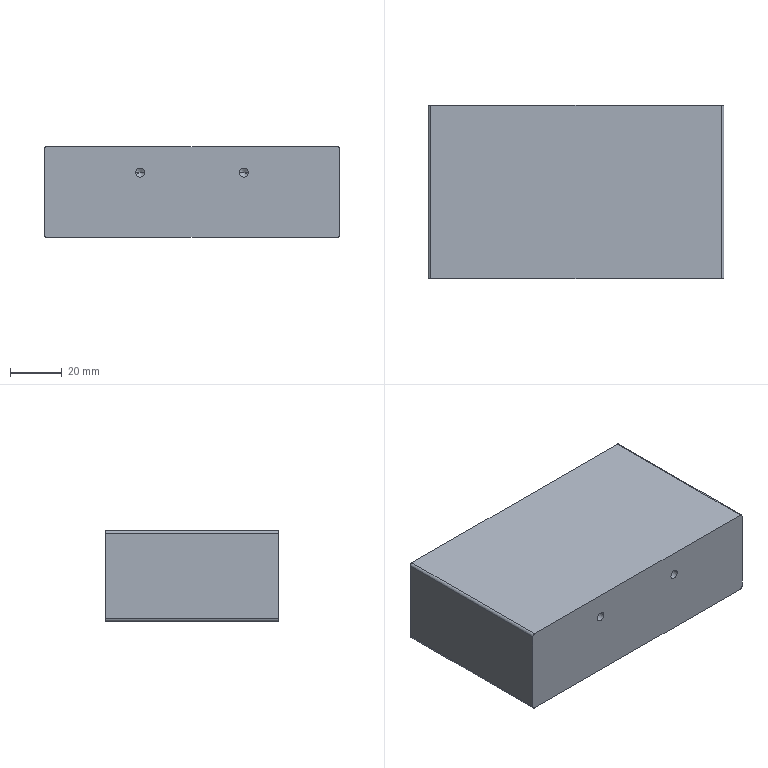Part | NX | 1 solid | 34 faces | box 114 x 67 x 35 mm | volume 266646 mm3 | cylinder 16 | cone 12 | plane 6 | commonest cylinder face diameters 3.5 x12 2 x4
STEP:
#1=CARTESIAN_POINT('',(57.,33.5,-1.));
#2=VERTEX_POINT('',#1);
#3=CARTESIAN_POINT('',(57.,33.5,-34.));
#4=VERTEX_POINT('',#3);
#5=CARTESIAN_POINT('',(57.,33.5,-1.));
#6=DIRECTION('',(0.,0.,-1.));
#7=VECTOR('',#6,1000.);
#8=LINE('',#5,#7);
#9=EDGE_CURVE('',#2,#4,#8,.T.);
#10=ORIENTED_EDGE('',*,*,#9,.T.);
#11=CARTESIAN_POINT('',(56.,33.5,-35.));
#12=VERTEX_POINT('',#11);
#13=CARTESIAN_POINT('',(56.,33.5,-34.));
#14=DIRECTION('',(0.,1.,0.));
#15=DIRECTION('',(1.,0.,0.));
#16=AXIS2_PLACEMENT_3D('',#13,#14,#15);
#17=CIRCLE('',#16,1.);
#18=EDGE_CURVE('',#4,#12,#17,.T.);
#19=ORIENTED_EDGE('',*,*,#18,.T.);
#20=CARTESIAN_POINT('',(-56.,33.5,-35.));
#21=VERTEX_POINT('',#20);
#22=CARTESIAN_POINT('',(56.,33.5,-35.));
#23=DIRECTION('',(-1.,0.,0.));
#24=VECTOR('',#23,1000.);
#25=LINE('',#22,#24);
#26=EDGE_CURVE('',#12,#21,#25,.T.);
#27=ORIENTED_EDGE('',*,*,#26,.T.);
#28=CARTESIAN_POINT('',(-57.,33.5,-34.));
#29=VERTEX_POINT('',#28);
#30=CARTESIAN_POINT('',(-56.,33.5,-34.));
#31=DIRECTION('',(0.,1.,0.));
#32=DIRECTION('',(0.,0.,-1.));
#33=AXIS2_PLACEMENT_3D('',#30,#31,#32);
#34=CIRCLE('',#33,1.);
#35=EDGE_CURVE('',#21,#29,#34,.T.);
#36=ORIENTED_EDGE('',*,*,#35,.T.);
#37=CARTESIAN_POINT('',(-57.,33.5,-1.));
#38=VERTEX_POINT('',#37);
#39=CARTESIAN_POINT('',(-57.,33.5,-34.));
#40=DIRECTION('',(0.,0.,1.));
#41=VECTOR('',#40,1000.);
#42=LINE('',#39,#41);
#43=EDGE_CURVE('',#29,#38,#42,.T.);
#44=ORIENTED_EDGE('',*,*,#43,.T.);
#45=CARTESIAN_POINT('',(-56.,33.5,0.));
#46=VERTEX_POINT('',#45);
#47=CARTESIAN_POINT('',(-56.,33.5,-1.));
#48=DIRECTION('',(0.,1.,0.));
#49=DIRECTION('',(-1.,0.,0.));
#50=AXIS2_PLACEMENT_3D('',#47,#48,#49);
#51=CIRCLE('',#50,1.);
#52=EDGE_CURVE('',#38,#46,#51,.T.);
#53=ORIENTED_EDGE('',*,*,#52,.T.);
#54=CARTESIAN_POINT('',(56.,33.5,0.));
#55=VERTEX_POINT('',#54);
#56=CARTESIAN_POINT('',(-56.,33.5,0.));
#57=DIRECTION('',(1.,0.,0.));
#58=VECTOR('',#57,1000.);
#59=LINE('',#56,#58);
#60=EDGE_CURVE('',#46,#55,#59,.T.);
#61=ORIENTED_EDGE('',*,*,#60,.T.);
#62=CARTESIAN_POINT('',(56.,33.5,-1.));
#63=DIRECTION('',(0.,1.,0.));
#64=DIRECTION('',(0.,0.,1.));
#65=AXIS2_PLACEMENT_3D('',#62,#63,#64);
#66=CIRCLE('',#65,1.);
#67=EDGE_CURVE('',#55,#2,#66,.T.);
#68=ORIENTED_EDGE('',*,*,#67,.T.);
#69=EDGE_LOOP('',(#10,#19,#27,#36,#44,#53,#61,#68));
#70=FACE_BOUND('',#69,.T.);
#71=CARTESIAN_POINT('',(15.75,33.5,-10.));
#72=VERTEX_POINT('',#71);
#73=CARTESIAN_POINT('',(19.25,33.5,-10.));
#74=VERTEX_POINT('',#73);
#75=CARTESIAN_POINT('',(17.5,33.5,-10.));
#76=DIRECTION('',(0.,1.,0.));
#77=DIRECTION('',(-1.,0.,0.));
#78=AXIS2_PLACEMENT_3D('',#75,#76,#77);
#79=CIRCLE('',#78,1.75);
#80=EDGE_CURVE('',#72,#74,#79,.T.);
#81=ORIENTED_EDGE('',*,*,#80,.F.);
#82=CARTESIAN_POINT('',(17.5,33.5,-10.));
#83=DIRECTION('',(0.,1.,0.));
#84=DIRECTION('',(1.,0.,0.));
#85=AXIS2_PLACEMENT_3D('',#82,#83,#84);
#86=CIRCLE('',#85,1.75);
#87=EDGE_CURVE('',#74,#72,#86,.T.);
#88=ORIENTED_EDGE('',*,*,#87,.F.);
#89=EDGE_LOOP('',(#81,#88));
#90=FACE_BOUND('',#89,.T.);
#91=CARTESIAN_POINT('',(50.75,33.5,-10.));
#92=VERTEX_POINT('',#91);
#93=CARTESIAN_POINT('',(54.25,33.5,-10.));
#94=VERTEX_POINT('',#93);
#95=CARTESIAN_POINT('',(52.5,33.5,-10.));
#96=DIRECTION('',(0.,1.,0.));
#97=DIRECTION('',(-1.,0.,0.));
#98=AXIS2_PLACEMENT_3D('',#95,#96,#97);
#99=CIRCLE('',#98,1.75);
#100=EDGE_CURVE('',#92,#94,#99,.T.);
#101=ORIENTED_EDGE('',*,*,#100,.F.);
#102=CARTESIAN_POINT('',(52.5,33.5,-10.));
#103=DIRECTION('',(0.,1.,0.));
#104=DIRECTION('',(1.,0.,0.));
#105=AXIS2_PLACEMENT_3D('',#102,#103,#104);
#106=CIRCLE('',#105,1.75);
#107=EDGE_CURVE('',#94,#92,#106,.T.);
#108=ORIENTED_EDGE('',*,*,#107,.F.);
#109=EDGE_LOOP('',(#101,#108));
#110=FACE_BOUND('',#109,.T.);
#111=CARTESIAN_POINT('',(-54.25,33.5,-10.));
#112=VERTEX_POINT('',#111);
#113=CARTESIAN_POINT('',(-50.75,33.5,-10.));
#114=VERTEX_POINT('',#113);
#115=CARTESIAN_POINT('',(-52.5,33.5,-10.));
#116=DIRECTION('',(0.,1.,0.));
#117=DIRECTION('',(-1.,0.,0.));
#118=AXIS2_PLACEMENT_3D('',#115,#116,#117);
#119=CIRCLE('',#118,1.75);
#120=EDGE_CURVE('',#112,#114,#119,.T.);
#121=ORIENTED_EDGE('',*,*,#120,.F.);
#122=CARTESIAN_POINT('',(-52.5,33.5,-10.));
#123=DIRECTION('',(0.,1.,0.));
#124=DIRECTION('',(1.,0.,0.));
#125=AXIS2_PLACEMENT_3D('',#122,#123,#124);
#126=CIRCLE('',#125,1.75);
#127=EDGE_CURVE('',#114,#112,#126,.T.);
#128=ORIENTED_EDGE('',*,*,#127,.F.);
#129=EDGE_LOOP('',(#121,#128));
#130=FACE_BOUND('',#129,.T.);
#131=CARTESIAN_POINT('',(-19.25,33.5,-10.));
#132=VERTEX_POINT('',#131);
#133=CARTESIAN_POINT('',(-15.75,33.5,-10.));
#134=VERTEX_POINT('',#133);
#135=CARTESIAN_POINT('',(-17.5,33.5,-10.));
#136=DIRECTION('',(0.,1.,0.));
#137=DIRECTION('',(-1.,0.,0.));
#138=AXIS2_PLACEMENT_3D('',#135,#136,#137);
#139=CIRCLE('',#138,1.75);
#140=EDGE_CURVE('',#132,#134,#139,.T.);
#141=ORIENTED_EDGE('',*,*,#140,.F.);
#142=CARTESIAN_POINT('',(-17.5,33.5,-10.));
#143=DIRECTION('',(0.,1.,0.));
#144=DIRECTION('',(1.,0.,0.));
#145=AXIS2_PLACEMENT_3D('',#142,#143,#144);
#146=CIRCLE('',#145,1.75);
#147=EDGE_CURVE('',#134,#132,#146,.T.);
#148=ORIENTED_EDGE('',*,*,#147,.F.);
#149=EDGE_LOOP('',(#141,#148));
#150=FACE_BOUND('',#149,.T.);
#151=CARTESIAN_POINT('',(0.,33.5,-10.));
#152=DIRECTION('',(0.,-1.,0.));
#153=DIRECTION('',(1.,0.,0.));
#154=AXIS2_PLACEMENT_3D('',#151,#152,#153);
#155=PLANE('',#154);
#156=ADVANCED_FACE('',(#70,#90,#110,#130,#150),#155,.F.);
#157=CARTESIAN_POINT('',(-19.25,23.,-10.));
#158=VERTEX_POINT('',#157);
#159=CARTESIAN_POINT('',(-19.25,33.5,-10.));
#160=DIRECTION('',(0.,-1.,0.));
#161=VECTOR('',#160,1000.);
#162=LINE('',#159,#161);
#163=EDGE_CURVE('',#158,#132,#162,.F.);
#164=ORIENTED_EDGE('',*,*,#163,.F.);
#165=CARTESIAN_POINT('',(-15.75,23.,-10.));
#166=VERTEX_POINT('',#165);
#167=CARTESIAN_POINT('',(-17.5,23.,-10.));
#168=DIRECTION('',(0.,-1.,0.));
#169=DIRECTION('',(-1.,0.,0.));
#170=AXIS2_PLACEMENT_3D('',#167,#168,#169);
#171=CIRCLE('',#170,1.75);
#172=EDGE_CURVE('',#158,#166,#171,.T.);
#173=ORIENTED_EDGE('',*,*,#172,.T.);
#174=CARTESIAN_POINT('',(-15.75,33.5,-10.));
#175=DIRECTION('',(0.,-1.,0.));
#176=VECTOR('',#175,1000.);
#177=LINE('',#174,#176);
#178=EDGE_CURVE('',#166,#134,#177,.F.);
#179=ORIENTED_EDGE('',*,*,#178,.T.);
#180=ORIENTED_EDGE('',*,*,#147,.T.);
#181=EDGE_LOOP('',(#164,#173,#179,#180));
#182=FACE_BOUND('',#181,.T.);
#183=CARTESIAN_POINT('',(-17.5,21.371,-10.));
#184=DIRECTION('',(0.,1.,0.));
#185=DIRECTION('',(-1.,0.,0.));
#186=AXIS2_PLACEMENT_3D('',#183,#184,#185);
#187=CYLINDRICAL_SURFACE('',#186,1.75);
#188=ADVANCED_FACE('',(#182),#187,.F.);
#189=ORIENTED_EDGE('',*,*,#178,.F.);
#190=CARTESIAN_POINT('',(-17.5,23.,-10.));
#191=DIRECTION('',(0.,-1.,0.));
#192=DIRECTION('',(1.,0.,0.));
#193=AXIS2_PLACEMENT_3D('',#190,#191,#192);
#194=CIRCLE('',#193,1.75);
#195=EDGE_CURVE('',#166,#158,#194,.T.);
#196=ORIENTED_EDGE('',*,*,#195,.T.);
#197=ORIENTED_EDGE('',*,*,#163,.T.);
#198=ORIENTED_EDGE('',*,*,#140,.T.);
#199=EDGE_LOOP('',(#189,#196,#197,#198));
#200=FACE_BOUND('',#199,.T.);
#201=CARTESIAN_POINT('',(-17.5,21.371,-10.));
#202=DIRECTION('',(0.,1.,0.));
#203=DIRECTION('',(-1.,0.,0.));
#204=AXIS2_PLACEMENT_3D('',#201,#202,#203);
#205=CYLINDRICAL_SURFACE('',#204,1.75);
#206=ADVANCED_FACE('',(#200),#205,.F.);
#207=CARTESIAN_POINT('',(-17.5,21.948,-10.));
#208=VERTEX_POINT('',#207);
#209=CARTESIAN_POINT('',(-19.25,23.,-10.));
#210=DIRECTION('',(0.8572,-0.515,0.));
#211=VECTOR('',#210,1000.);
#212=LINE('',#209,#211);
#213=EDGE_CURVE('',#158,#208,#212,.T.);
#214=ORIENTED_EDGE('',*,*,#213,.F.);
#215=ORIENTED_EDGE('',*,*,#195,.F.);
#216=CARTESIAN_POINT('',(-17.5,21.948,-10.));
#217=DIRECTION('',(0.8572,0.515,0.));
#218=VECTOR('',#217,1000.);
#219=LINE('',#216,#218);
#220=EDGE_CURVE('',#208,#166,#219,.T.);
#221=ORIENTED_EDGE('',*,*,#220,.F.);
#222=EDGE_LOOP('',(#214,#215,#221));
#223=FACE_BOUND('',#222,.T.);
#224=CARTESIAN_POINT('',(-17.5,22.474,-10.));
#225=DIRECTION('',(0.,1.,0.));
#226=DIRECTION('',(-1.,0.,0.));
#227=AXIS2_PLACEMENT_3D('',#224,#225,#226);
#228=CONICAL_SURFACE('',#227,0.875,1.03);
#229=ADVANCED_FACE('',(#223),#228,.F.);
#230=ORIENTED_EDGE('',*,*,#172,.F.);
#231=ORIENTED_EDGE('',*,*,#213,.T.);
#232=ORIENTED_EDGE('',*,*,#220,.T.);
#233=EDGE_LOOP('',(#230,#231,#232));
#234=FACE_BOUND('',#233,.T.);
#235=CARTESIAN_POINT('',(-17.5,22.474,-10.));
#236=DIRECTION('',(0.,1.,0.));
#237=DIRECTION('',(-1.,0.,0.));
#238=AXIS2_PLACEMENT_3D('',#235,#236,#237);
#239=CONICAL_SURFACE('',#238,0.875,1.03);
#240=ADVANCED_FACE('',(#234),#239,.F.);
#241=CARTESIAN_POINT('',(15.75,23.,-10.));
#242=VERTEX_POINT('',#241);
#243=CARTESIAN_POINT('',(15.75,33.5,-10.));
#244=DIRECTION('',(0.,-1.,0.));
#245=VECTOR('',#244,1000.);
#246=LINE('',#243,#245);
#247=EDGE_CURVE('',#242,#72,#246,.F.);
#248=ORIENTED_EDGE('',*,*,#247,.F.);
#249=CARTESIAN_POINT('',(19.25,23.,-10.));
#250=VERTEX_POINT('',#249);
#251=CARTESIAN_POINT('',(17.5,23.,-10.));
#252=DIRECTION('',(0.,-1.,0.));
#253=DIRECTION('',(-1.,0.,0.));
#254=AXIS2_PLACEMENT_3D('',#251,#252,#253);
#255=CIRCLE('',#254,1.75);
#256=EDGE_CURVE('',#242,#250,#255,.T.);
#257=ORIENTED_EDGE('',*,*,#256,.T.);
#258=CARTESIAN_POINT('',(19.25,33.5,-10.));
#259=DIRECTION('',(0.,-1.,0.));
#260=VECTOR('',#259,1000.);
#261=LINE('',#258,#260);
#262=EDGE_CURVE('',#250,#74,#261,.F.);
#263=ORIENTED_EDGE('',*,*,#262,.T.);
#264=ORIENTED_EDGE('',*,*,#87,.T.);
#265=EDGE_LOOP('',(#248,#257,#263,#264));
#266=FACE_BOUND('',#265,.T.);
#267=CARTESIAN_POINT('',(17.5,21.371,-10.));
#268=DIRECTION('',(0.,1.,0.));
#269=DIRECTION('',(-1.,0.,0.));
#270=AXIS2_PLACEMENT_3D('',#267,#268,#269);
#271=CYLINDRICAL_SURFACE('',#270,1.75);
#272=ADVANCED_FACE('',(#266),#271,.F.);
#273=ORIENTED_EDGE('',*,*,#262,.F.);
#274=CARTESIAN_POINT('',(17.5,23.,-10.));
#275=DIRECTION('',(0.,-1.,0.));
#276=DIRECTION('',(1.,0.,0.));
#277=AXIS2_PLACEMENT_3D('',#274,#275,#276);
#278=CIRCLE('',#277,1.75);
#279=EDGE_CURVE('',#250,#242,#278,.T.);
#280=ORIENTED_EDGE('',*,*,#279,.T.);
#281=ORIENTED_EDGE('',*,*,#247,.T.);
#282=ORIENTED_EDGE('',*,*,#80,.T.);
#283=EDGE_LOOP('',(#273,#280,#281,#282));
#284=FACE_BOUND('',#283,.T.);
#285=CARTESIAN_POINT('',(17.5,21.371,-10.));
#286=DIRECTION('',(0.,1.,0.));
#287=DIRECTION('',(-1.,0.,0.));
#288=AXIS2_PLACEMENT_3D('',#285,#286,#287);
#289=CYLINDRICAL_SURFACE('',#288,1.75);
#290=ADVANCED_FACE('',(#284),#289,.F.);
#291=CARTESIAN_POINT('',(17.5,21.948,-10.));
#292=VERTEX_POINT('',#291);
#293=CARTESIAN_POINT('',(15.75,23.,-10.));
#294=DIRECTION('',(0.8572,-0.515,0.));
#295=VECTOR('',#294,1000.);
#296=LINE('',#293,#295);
#297=EDGE_CURVE('',#292,#242,#296,.F.);
#298=ORIENTED_EDGE('',*,*,#297,.T.);
#299=ORIENTED_EDGE('',*,*,#279,.F.);
#300=CARTESIAN_POINT('',(19.25,23.,-10.));
#301=DIRECTION('',(-0.8572,-0.515,0.));
#302=VECTOR('',#301,1000.);
#303=LINE('',#300,#302);
#304=EDGE_CURVE('',#292,#250,#303,.F.);
#305=ORIENTED_EDGE('',*,*,#304,.F.);
#306=EDGE_LOOP('',(#298,#299,#305));
#307=FACE_BOUND('',#306,.T.);
#308=CARTESIAN_POINT('',(17.5,22.474,-10.));
#309=DIRECTION('',(0.,1.,0.));
#310=DIRECTION('',(-1.,0.,0.));
#311=AXIS2_PLACEMENT_3D('',#308,#309,#310);
#312=CONICAL_SURFACE('',#311,0.875,1.03);
#313=ADVANCED_FACE('',(#307),#312,.F.);
#314=ORIENTED_EDGE('',*,*,#256,.F.);
#315=ORIENTED_EDGE('',*,*,#297,.F.);
#316=ORIENTED_EDGE('',*,*,#304,.T.);
#317=EDGE_LOOP('',(#314,#315,#316));
#318=FACE_BOUND('',#317,.T.);
#319=CARTESIAN_POINT('',(17.5,22.474,-10.));
#320=DIRECTION('',(0.,1.,0.));
#321=DIRECTION('',(-1.,0.,0.));
#322=AXIS2_PLACEMENT_3D('',#319,#320,#321);
#323=CONICAL_SURFACE('',#322,0.875,1.03);
#324=ADVANCED_FACE('',(#318),#323,.F.);
#325=CARTESIAN_POINT('',(50.75,23.,-10.));
#326=VERTEX_POINT('',#325);
#327=CARTESIAN_POINT('',(50.75,33.5,-10.));
#328=DIRECTION('',(0.,-1.,0.));
#329=VECTOR('',#328,1000.);
#330=LINE('',#327,#329);
#331=EDGE_CURVE('',#326,#92,#330,.F.);
#332=ORIENTED_EDGE('',*,*,#331,.F.);
#333=CARTESIAN_POINT('',(54.25,23.,-10.));
#334=VERTEX_POINT('',#333);
#335=CARTESIAN_POINT('',(52.5,23.,-10.));
#336=DIRECTION('',(0.,-1.,0.));
#337=DIRECTION('',(-1.,0.,0.));
#338=AXIS2_PLACEMENT_3D('',#335,#336,#337);
#339=CIRCLE('',#338,1.75);
#340=EDGE_CURVE('',#326,#334,#339,.T.);
#341=ORIENTED_EDGE('',*,*,#340,.T.);
#342=CARTESIAN_POINT('',(54.25,33.5,-10.));
#343=DIRECTION('',(0.,-1.,0.));
#344=VECTOR('',#343,1000.);
#345=LINE('',#342,#344);
#346=EDGE_CURVE('',#334,#94,#345,.F.);
#347=ORIENTED_EDGE('',*,*,#346,.T.);
#348=ORIENTED_EDGE('',*,*,#107,.T.);
#349=EDGE_LOOP('',(#332,#341,#347,#348));
#350=FACE_BOUND('',#349,.T.);
#351=CARTESIAN_POINT('',(52.5,21.371,-10.));
#352=DIRECTION('',(0.,1.,0.));
#353=DIRECTION('',(-1.,0.,0.));
#354=AXIS2_PLACEMENT_3D('',#351,#352,#353);
#355=CYLINDRICAL_SURFACE('',#354,1.75);
#356=ADVANCED_FACE('',(#350),#355,.F.);
#357=ORIENTED_EDGE('',*,*,#346,.F.);
#358=CARTESIAN_POINT('',(52.5,23.,-10.));
#359=DIRECTION('',(0.,-1.,0.));
#360=DIRECTION('',(1.,0.,0.));
#361=AXIS2_PLACEMENT_3D('',#358,#359,#360);
#362=CIRCLE('',#361,1.75);
#363=EDGE_CURVE('',#334,#326,#362,.T.);
#364=ORIENTED_EDGE('',*,*,#363,.T.);
#365=ORIENTED_EDGE('',*,*,#331,.T.);
#366=ORIENTED_EDGE('',*,*,#100,.T.);
#367=EDGE_LOOP('',(#357,#364,#365,#366));
#368=FACE_BOUND('',#367,.T.);
#369=CARTESIAN_POINT('',(52.5,21.371,-10.));
#370=DIRECTION('',(0.,1.,0.));
#371=DIRECTION('',(-1.,0.,0.));
#372=AXIS2_PLACEMENT_3D('',#369,#370,#371);
#373=CYLINDRICAL_SURFACE('',#372,1.75);
#374=ADVANCED_FACE('',(#368),#373,.F.);
#375=CARTESIAN_POINT('',(52.5,21.948,-10.));
#376=VERTEX_POINT('',#375);
#377=CARTESIAN_POINT('',(50.75,23.,-10.));
#378=DIRECTION('',(0.8572,-0.515,0.));
#379=VECTOR('',#378,1000.);
#380=LINE('',#377,#379);
#381=EDGE_CURVE('',#376,#326,#380,.F.);
#382=ORIENTED_EDGE('',*,*,#381,.T.);
#383=ORIENTED_EDGE('',*,*,#363,.F.);
#384=CARTESIAN_POINT('',(54.25,23.,-10.));
#385=DIRECTION('',(-0.8572,-0.515,0.));
#386=VECTOR('',#385,1000.);
#387=LINE('',#384,#386);
#388=EDGE_CURVE('',#376,#334,#387,.F.);
#389=ORIENTED_EDGE('',*,*,#388,.F.);
#390=EDGE_LOOP('',(#382,#383,#389));
#391=FACE_BOUND('',#390,.T.);
#392=CARTESIAN_POINT('',(52.5,22.474,-10.));
#393=DIRECTION('',(0.,1.,0.));
#394=DIRECTION('',(-1.,0.,0.));
#395=AXIS2_PLACEMENT_3D('',#392,#393,#394);
#396=CONICAL_SURFACE('',#395,0.875,1.03);
#397=ADVANCED_FACE('',(#391),#396,.F.);
#398=ORIENTED_EDGE('',*,*,#340,.F.);
#399=ORIENTED_EDGE('',*,*,#381,.F.);
#400=ORIENTED_EDGE('',*,*,#388,.T.);
#401=EDGE_LOOP('',(#398,#399,#400));
#402=FACE_BOUND('',#401,.T.);
#403=CARTESIAN_POINT('',(52.5,22.474,-10.));
#404=DIRECTION('',(0.,1.,0.));
#405=DIRECTION('',(-1.,0.,0.));
#406=AXIS2_PLACEMENT_3D('',#403,#404,#405);
#407=CONICAL_SURFACE('',#406,0.875,1.03);
#408=ADVANCED_FACE('',(#402),#407,.F.);
#409=CARTESIAN_POINT('',(-54.25,23.,-10.));
#410=VERTEX_POINT('',#409);
#411=CARTESIAN_POINT('',(-54.25,33.5,-10.));
#412=DIRECTION('',(0.,-1.,0.));
#413=VECTOR('',#412,1000.);
#414=LINE('',#411,#413);
#415=EDGE_CURVE('',#410,#112,#414,.F.);
#416=ORIENTED_EDGE('',*,*,#415,.F.);
#417=CARTESIAN_POINT('',(-50.75,23.,-10.));
#418=VERTEX_POINT('',#417);
#419=CARTESIAN_POINT('',(-52.5,23.,-10.));
#420=DIRECTION('',(0.,-1.,0.));
#421=DIRECTION('',(-1.,0.,0.));
#422=AXIS2_PLACEMENT_3D('',#419,#420,#421);
#423=CIRCLE('',#422,1.75);
#424=EDGE_CURVE('',#410,#418,#423,.T.);
#425=ORIENTED_EDGE('',*,*,#424,.T.);
#426=CARTESIAN_POINT('',(-50.75,33.5,-10.));
#427=DIRECTION('',(0.,-1.,0.));
#428=VECTOR('',#427,1000.);
#429=LINE('',#426,#428);
#430=EDGE_CURVE('',#418,#114,#429,.F.);
#431=ORIENTED_EDGE('',*,*,#430,.T.);
#432=ORIENTED_EDGE('',*,*,#127,.T.);
#433=EDGE_LOOP('',(#416,#425,#431,#432));
#434=FACE_BOUND('',#433,.T.);
#435=CARTESIAN_POINT('',(-52.5,21.371,-10.));
#436=DIRECTION('',(0.,1.,0.));
#437=DIRECTION('',(-1.,0.,0.));
#438=AXIS2_PLACEMENT_3D('',#435,#436,#437);
#439=CYLINDRICAL_SURFACE('',#438,1.75);
#440=ADVANCED_FACE('',(#434),#439,.F.);
#441=ORIENTED_EDGE('',*,*,#430,.F.);
#442=CARTESIAN_POINT('',(-52.5,23.,-10.));
#443=DIRECTION('',(0.,-1.,0.));
#444=DIRECTION('',(1.,0.,0.));
#445=AXIS2_PLACEMENT_3D('',#442,#443,#444);
#446=CIRCLE('',#445,1.75);
#447=EDGE_CURVE('',#418,#410,#446,.T.);
#448=ORIENTED_EDGE('',*,*,#447,.T.);
#449=ORIENTED_EDGE('',*,*,#415,.T.);
#450=ORIENTED_EDGE('',*,*,#120,.T.);
#451=EDGE_LOOP('',(#441,#448,#449,#450));
#452=FACE_BOUND('',#451,.T.);
#453=CARTESIAN_POINT('',(-52.5,21.371,-10.));
#454=DIRECTION('',(0.,1.,0.));
#455=DIRECTION('',(-1.,0.,0.));
#456=AXIS2_PLACEMENT_3D('',#453,#454,#455);
#457=CYLINDRICAL_SURFACE('',#456,1.75);
#458=ADVANCED_FACE('',(#452),#457,.F.);
#459=CARTESIAN_POINT('',(-52.5,21.948,-10.));
#460=VERTEX_POINT('',#459);
#461=CARTESIAN_POINT('',(-54.25,23.,-10.));
#462=DIRECTION('',(0.8572,-0.515,0.));
#463=VECTOR('',#462,1000.);
#464=LINE('',#461,#463);
#465=EDGE_CURVE('',#410,#460,#464,.T.);
#466=ORIENTED_EDGE('',*,*,#465,.F.);
#467=ORIENTED_EDGE('',*,*,#447,.F.);
#468=CARTESIAN_POINT('',(-52.5,21.948,-10.));
#469=DIRECTION('',(0.8572,0.515,0.));
#470=VECTOR('',#469,1000.);
#471=LINE('',#468,#470);
#472=EDGE_CURVE('',#460,#418,#471,.T.);
#473=ORIENTED_EDGE('',*,*,#472,.F.);
#474=EDGE_LOOP('',(#466,#467,#473));
#475=FACE_BOUND('',#474,.T.);
#476=CARTESIAN_POINT('',(-52.5,22.474,-10.));
#477=DIRECTION('',(0.,1.,0.));
#478=DIRECTION('',(-1.,0.,0.));
#479=AXIS2_PLACEMENT_3D('',#476,#477,#478);
#480=CONICAL_SURFACE('',#479,0.875,1.03);
#481=ADVANCED_FACE('',(#475),#480,.F.);
#482=ORIENTED_EDGE('',*,*,#424,.F.);
#483=ORIENTED_EDGE('',*,*,#465,.T.);
#484=ORIENTED_EDGE('',*,*,#472,.T.);
#485=EDGE_LOOP('',(#482,#483,#484));
#486=FACE_BOUND('',#485,.T.);
#487=CARTESIAN_POINT('',(-52.5,22.474,-10.));
#488=DIRECTION('',(0.,1.,0.));
#489=DIRECTION('',(-1.,0.,0.));
#490=AXIS2_PLACEMENT_3D('',#487,#488,#489);
#491=CONICAL_SURFACE('',#490,0.875,1.03);
#492=ADVANCED_FACE('',(#486),#491,.F.);
#493=CARTESIAN_POINT('',(56.,-33.5,0.));
#494=VERTEX_POINT('',#493);
#495=CARTESIAN_POINT('',(56.,-33.5,0.));
#496=DIRECTION('',(0.,1.,0.));
#497=VECTOR('',#496,1000.);
#498=LINE('',#495,#497);
#499=EDGE_CURVE('',#494,#55,#498,.T.);
#500=ORIENTED_EDGE('',*,*,#499,.F.);
#501=CARTESIAN_POINT('',(57.,-33.5,-1.));
#502=VERTEX_POINT('',#501);
#503=CARTESIAN_POINT('',(56.,-33.5,-1.));
#504=DIRECTION('',(0.,-1.,0.));
#505=DIRECTION('',(1.,0.,0.));
#506=AXIS2_PLACEMENT_3D('',#503,#504,#505);
#507=CIRCLE('',#506,1.);
#508=EDGE_CURVE('',#502,#494,#507,.T.);
#509=ORIENTED_EDGE('',*,*,#508,.F.);
#510=CARTESIAN_POINT('',(57.,-33.5,-1.));
#511=DIRECTION('',(0.,1.,0.));
#512=VECTOR('',#511,1000.);
#513=LINE('',#510,#512);
#514=EDGE_CURVE('',#502,#2,#513,.T.);
#515=ORIENTED_EDGE('',*,*,#514,.T.);
#516=ORIENTED_EDGE('',*,*,#67,.F.);
#517=EDGE_LOOP('',(#500,#509,#515,#516));
#518=FACE_BOUND('',#517,.T.);
#519=CARTESIAN_POINT('',(56.,-120.841,-1.));
#520=DIRECTION('',(0.,1.,0.));
#521=DIRECTION('',(0.,0.,-1.));
#522=AXIS2_PLACEMENT_3D('',#519,#520,#521);
#523=CYLINDRICAL_SURFACE('',#522,1.);
#524=ADVANCED_FACE('',(#518),#523,.T.);
#525=CARTESIAN_POINT('',(57.,-33.5,-34.));
#526=VERTEX_POINT('',#525);
#527=CARTESIAN_POINT('',(57.,-33.5,-34.));
#528=DIRECTION('',(0.,0.,1.));
#529=VECTOR('',#528,1000.);
#530=LINE('',#527,#529);
#531=EDGE_CURVE('',#526,#502,#530,.T.);
#532=ORIENTED_EDGE('',*,*,#531,.F.);
#533=CARTESIAN_POINT('',(57.,-33.5,-34.));
#534=DIRECTION('',(0.,1.,0.));
#535=VECTOR('',#534,1000.);
#536=LINE('',#533,#535);
#537=EDGE_CURVE('',#526,#4,#536,.T.);
#538=ORIENTED_EDGE('',*,*,#537,.T.);
#539=ORIENTED_EDGE('',*,*,#9,.F.);
#540=ORIENTED_EDGE('',*,*,#514,.F.);
#541=EDGE_LOOP('',(#532,#538,#539,#540));
#542=FACE_BOUND('',#541,.T.);
#543=CARTESIAN_POINT('',(57.,33.5,-20.));
#544=DIRECTION('',(1.,0.,0.));
#545=DIRECTION('',(0.,0.,-1.));
#546=AXIS2_PLACEMENT_3D('',#543,#544,#545);
#547=PLANE('',#546);
#548=ADVANCED_FACE('',(#542),#547,.T.);
#549=ORIENTED_EDGE('',*,*,#537,.F.);
#550=CARTESIAN_POINT('',(56.,-33.5,-35.));
#551=VERTEX_POINT('',#550);
#552=CARTESIAN_POINT('',(56.,-33.5,-34.));
#553=DIRECTION('',(0.,-1.,0.));
#554=DIRECTION('',(0.,0.,-1.));
#555=AXIS2_PLACEMENT_3D('',#552,#553,#554);
#556=CIRCLE('',#555,1.);
#557=EDGE_CURVE('',#551,#526,#556,.T.);
#558=ORIENTED_EDGE('',*,*,#557,.F.);
#559=CARTESIAN_POINT('',(56.,-33.5,-35.));
#560=DIRECTION('',(0.,1.,0.));
#561=VECTOR('',#560,1000.);
#562=LINE('',#559,#561);
#563=EDGE_CURVE('',#551,#12,#562,.T.);
#564=ORIENTED_EDGE('',*,*,#563,.T.);
#565=ORIENTED_EDGE('',*,*,#18,.F.);
#566=EDGE_LOOP('',(#549,#558,#564,#565));
#567=FACE_BOUND('',#566,.T.);
#568=CARTESIAN_POINT('',(56.,-120.841,-34.));
#569=DIRECTION('',(0.,1.,0.));
#570=DIRECTION('',(-1.,0.,0.));
#571=AXIS2_PLACEMENT_3D('',#568,#569,#570);
#572=CYLINDRICAL_SURFACE('',#571,1.);
#573=ADVANCED_FACE('',(#567),#572,.T.);
#574=CARTESIAN_POINT('',(-56.,-33.5,-35.));
#575=VERTEX_POINT('',#574);
#576=CARTESIAN_POINT('',(-56.,-33.5,-35.));
#577=DIRECTION('',(1.,0.,0.));
#578=VECTOR('',#577,1000.);
#579=LINE('',#576,#578);
#580=EDGE_CURVE('',#575,#551,#579,.T.);
#581=ORIENTED_EDGE('',*,*,#580,.F.);
#582=CARTESIAN_POINT('',(-56.,-33.5,-35.));
#583=DIRECTION('',(0.,1.,0.));
#584=VECTOR('',#583,1000.);
#585=LINE('',#582,#584);
#586=EDGE_CURVE('',#575,#21,#585,.T.);
#587=ORIENTED_EDGE('',*,*,#586,.T.);
#588=ORIENTED_EDGE('',*,*,#26,.F.);
#589=ORIENTED_EDGE('',*,*,#563,.F.);
#590=EDGE_LOOP('',(#581,#587,#588,#589));
#591=FACE_BOUND('',#590,.T.);
#592=CARTESIAN_POINT('',(-60.,33.5,-35.));
#593=DIRECTION('',(0.,0.,-1.));
#594=DIRECTION('',(-1.,0.,0.));
#595=AXIS2_PLACEMENT_3D('',#592,#593,#594);
#596=PLANE('',#595);
#597=ADVANCED_FACE('',(#591),#596,.T.);
#598=ORIENTED_EDGE('',*,*,#586,.F.);
#599=CARTESIAN_POINT('',(-57.,-33.5,-34.));
#600=VERTEX_POINT('',#599);
#601=CARTESIAN_POINT('',(-56.,-33.5,-34.));
#602=DIRECTION('',(0.,-1.,0.));
#603=DIRECTION('',(-1.,0.,0.));
#604=AXIS2_PLACEMENT_3D('',#601,#602,#603);
#605=CIRCLE('',#604,1.);
#606=EDGE_CURVE('',#600,#575,#605,.T.);
#607=ORIENTED_EDGE('',*,*,#606,.F.);
#608=CARTESIAN_POINT('',(-57.,-33.5,-34.));
#609=DIRECTION('',(0.,1.,0.));
#610=VECTOR('',#609,1000.);
#611=LINE('',#608,#610);
#612=EDGE_CURVE('',#600,#29,#611,.T.);
#613=ORIENTED_EDGE('',*,*,#612,.T.);
#614=ORIENTED_EDGE('',*,*,#35,.F.);
#615=EDGE_LOOP('',(#598,#607,#613,#614));
#616=FACE_BOUND('',#615,.T.);
#617=CARTESIAN_POINT('',(-56.,-120.841,-34.));
#618=DIRECTION('',(0.,1.,0.));
#619=DIRECTION('',(0.,0.,1.));
#620=AXIS2_PLACEMENT_3D('',#617,#618,#619);
#621=CYLINDRICAL_SURFACE('',#620,1.);
#622=ADVANCED_FACE('',(#616),#621,.T.);
#623=ORIENTED_EDGE('',*,*,#43,.F.);
#624=ORIENTED_EDGE('',*,*,#612,.F.);
#625=CARTESIAN_POINT('',(-57.,-33.5,-1.));
#626=VERTEX_POINT('',#625);
#627=CARTESIAN_POINT('',(-57.,-33.5,-34.));
#628=DIRECTION('',(0.,0.,1.));
#629=VECTOR('',#628,1000.);
#630=LINE('',#627,#629);
#631=EDGE_CURVE('',#600,#626,#630,.T.);
#632=ORIENTED_EDGE('',*,*,#631,.T.);
#633=CARTESIAN_POINT('',(-57.,-33.5,-1.));
#634=DIRECTION('',(0.,1.,0.));
#635=VECTOR('',#634,1000.);
#636=LINE('',#633,#635);
#637=EDGE_CURVE('',#626,#38,#636,.T.);
#638=ORIENTED_EDGE('',*,*,#637,.T.);
#639=EDGE_LOOP('',(#623,#624,#632,#638));
#640=FACE_BOUND('',#639,.T.);
#641=CARTESIAN_POINT('',(-57.,33.5,0.));
#642=DIRECTION('',(-1.,0.,0.));
#643=DIRECTION('',(0.,0.,1.));
#644=AXIS2_PLACEMENT_3D('',#641,#642,#643);
#645=PLANE('',#644);
#646=ADVANCED_FACE('',(#640),#645,.T.);
#647=ORIENTED_EDGE('',*,*,#637,.F.);
#648=CARTESIAN_POINT('',(-56.,-33.5,0.));
#649=VERTEX_POINT('',#648);
#650=CARTESIAN_POINT('',(-56.,-33.5,-1.));
#651=DIRECTION('',(0.,-1.,0.));
#652=DIRECTION('',(0.,0.,1.));
#653=AXIS2_PLACEMENT_3D('',#650,#651,#652);
#654=CIRCLE('',#653,1.);
#655=EDGE_CURVE('',#649,#626,#654,.T.);
#656=ORIENTED_EDGE('',*,*,#655,.F.);
#657=CARTESIAN_POINT('',(-56.,-33.5,0.));
#658=DIRECTION('',(0.,1.,0.));
#659=VECTOR('',#658,1000.);
#660=LINE('',#657,#659);
#661=EDGE_CURVE('',#649,#46,#660,.T.);
#662=ORIENTED_EDGE('',*,*,#661,.T.);
#663=ORIENTED_EDGE('',*,*,#52,.F.);
#664=EDGE_LOOP('',(#647,#656,#662,#663));
#665=FACE_BOUND('',#664,.T.);
#666=CARTESIAN_POINT('',(-56.,-120.841,-1.));
#667=DIRECTION('',(0.,1.,0.));
#668=DIRECTION('',(1.,0.,0.));
#669=AXIS2_PLACEMENT_3D('',#666,#667,#668);
#670=CYLINDRICAL_SURFACE('',#669,1.);
#671=ADVANCED_FACE('',(#665),#670,.T.);
#672=ORIENTED_EDGE('',*,*,#60,.F.);
#673=ORIENTED_EDGE('',*,*,#661,.F.);
#674=CARTESIAN_POINT('',(56.,-33.5,0.));
#675=DIRECTION('',(-1.,0.,0.));
#676=VECTOR('',#675,1000.);
#677=LINE('',#674,#676);
#678=EDGE_CURVE('',#494,#649,#677,.T.);
#679=ORIENTED_EDGE('',*,*,#678,.F.);
#680=ORIENTED_EDGE('',*,*,#499,.T.);
#681=EDGE_LOOP('',(#672,#673,#679,#680));
#682=FACE_BOUND('',#681,.T.);
#683=CARTESIAN_POINT('',(60.,33.5,0.));
#684=DIRECTION('',(0.,0.,1.));
#685=DIRECTION('',(1.,0.,0.));
#686=AXIS2_PLACEMENT_3D('',#683,#684,#685);
#687=PLANE('',#686);
#688=ADVANCED_FACE('',(#682),#687,.T.);
#689=ORIENTED_EDGE('',*,*,#678,.T.);
#690=ORIENTED_EDGE('',*,*,#655,.T.);
#691=ORIENTED_EDGE('',*,*,#631,.F.);
#692=ORIENTED_EDGE('',*,*,#606,.T.);
#693=ORIENTED_EDGE('',*,*,#580,.T.);
#694=ORIENTED_EDGE('',*,*,#557,.T.);
#695=ORIENTED_EDGE('',*,*,#531,.T.);
#696=ORIENTED_EDGE('',*,*,#508,.T.);
#697=EDGE_LOOP('',(#689,#690,#691,#692,#693,#694,#695,#696));
#698=FACE_BOUND('',#697,.T.);
#699=CARTESIAN_POINT('',(-18.25,-33.5,-10.));
#700=VERTEX_POINT('',#699);
#701=CARTESIAN_POINT('',(-21.75,-33.5,-10.));
#702=VERTEX_POINT('',#701);
#703=CARTESIAN_POINT('',(-20.,-33.5,-10.));
#704=DIRECTION('',(0.,-1.,0.));
#705=DIRECTION('',(1.,0.,0.));
#706=AXIS2_PLACEMENT_3D('',#703,#704,#705);
#707=CIRCLE('',#706,1.75);
#708=EDGE_CURVE('',#700,#702,#707,.T.);
#709=ORIENTED_EDGE('',*,*,#708,.F.);
#710=CARTESIAN_POINT('',(-20.,-33.5,-10.));
#711=DIRECTION('',(0.,-1.,0.));
#712=DIRECTION('',(-1.,0.,0.));
#713=AXIS2_PLACEMENT_3D('',#710,#711,#712);
#714=CIRCLE('',#713,1.75);
#715=EDGE_CURVE('',#702,#700,#714,.T.);
#716=ORIENTED_EDGE('',*,*,#715,.F.);
#717=EDGE_LOOP('',(#709,#716));
#718=FACE_BOUND('',#717,.T.);
#719=CARTESIAN_POINT('',(21.75,-33.5,-10.));
#720=VERTEX_POINT('',#719);
#721=CARTESIAN_POINT('',(18.25,-33.5,-10.));
#722=VERTEX_POINT('',#721);
#723=CARTESIAN_POINT('',(20.,-33.5,-10.));
#724=DIRECTION('',(0.,-1.,0.));
#725=DIRECTION('',(1.,0.,0.));
#726=AXIS2_PLACEMENT_3D('',#723,#724,#725);
#727=CIRCLE('',#726,1.75);
#728=EDGE_CURVE('',#720,#722,#727,.T.);
#729=ORIENTED_EDGE('',*,*,#728,.F.);
#730=CARTESIAN_POINT('',(20.,-33.5,-10.));
#731=DIRECTION('',(0.,-1.,0.));
#732=DIRECTION('',(-1.,0.,0.));
#733=AXIS2_PLACEMENT_3D('',#730,#731,#732);
#734=CIRCLE('',#733,1.75);
#735=EDGE_CURVE('',#722,#720,#734,.T.);
#736=ORIENTED_EDGE('',*,*,#735,.F.);
#737=EDGE_LOOP('',(#729,#736));
#738=FACE_BOUND('',#737,.T.);
#739=CARTESIAN_POINT('',(0.,-33.5,-10.));
#740=DIRECTION('',(0.,-1.,0.));
#741=DIRECTION('',(1.,0.,0.));
#742=AXIS2_PLACEMENT_3D('',#739,#740,#741);
#743=PLANE('',#742);
#744=ADVANCED_FACE('',(#698,#718,#738),#743,.T.);
#745=CARTESIAN_POINT('',(21.75,-23.,-10.));
#746=VERTEX_POINT('',#745);
#747=CARTESIAN_POINT('',(21.75,-33.5,-10.));
#748=DIRECTION('',(0.,1.,0.));
#749=VECTOR('',#748,1000.);
#750=LINE('',#747,#749);
#751=EDGE_CURVE('',#746,#720,#750,.F.);
#752=ORIENTED_EDGE('',*,*,#751,.F.);
#753=CARTESIAN_POINT('',(18.25,-23.,-10.));
#754=VERTEX_POINT('',#753);
#755=CARTESIAN_POINT('',(20.,-23.,-10.));
#756=DIRECTION('',(0.,1.,0.));
#757=DIRECTION('',(1.,0.,0.));
#758=AXIS2_PLACEMENT_3D('',#755,#756,#757);
#759=CIRCLE('',#758,1.75);
#760=EDGE_CURVE('',#746,#754,#759,.T.);
#761=ORIENTED_EDGE('',*,*,#760,.T.);
#762=CARTESIAN_POINT('',(18.25,-33.5,-10.));
#763=DIRECTION('',(0.,1.,0.));
#764=VECTOR('',#763,1000.);
#765=LINE('',#762,#764);
#766=EDGE_CURVE('',#754,#722,#765,.F.);
#767=ORIENTED_EDGE('',*,*,#766,.T.);
#768=ORIENTED_EDGE('',*,*,#735,.T.);
#769=EDGE_LOOP('',(#752,#761,#767,#768));
#770=FACE_BOUND('',#769,.T.);
#771=CARTESIAN_POINT('',(20.,-21.371,-10.));
#772=DIRECTION('',(0.,-1.,0.));
#773=DIRECTION('',(1.,0.,0.));
#774=AXIS2_PLACEMENT_3D('',#771,#772,#773);
#775=CYLINDRICAL_SURFACE('',#774,1.75);
#776=ADVANCED_FACE('',(#770),#775,.F.);
#777=ORIENTED_EDGE('',*,*,#766,.F.);
#778=CARTESIAN_POINT('',(20.,-23.,-10.));
#779=DIRECTION('',(0.,1.,0.));
#780=DIRECTION('',(-1.,0.,0.));
#781=AXIS2_PLACEMENT_3D('',#778,#779,#780);
#782=CIRCLE('',#781,1.75);
#783=EDGE_CURVE('',#754,#746,#782,.T.);
#784=ORIENTED_EDGE('',*,*,#783,.T.);
#785=ORIENTED_EDGE('',*,*,#751,.T.);
#786=ORIENTED_EDGE('',*,*,#728,.T.);
#787=EDGE_LOOP('',(#777,#784,#785,#786));
#788=FACE_BOUND('',#787,.T.);
#789=CARTESIAN_POINT('',(20.,-21.371,-10.));
#790=DIRECTION('',(0.,-1.,0.));
#791=DIRECTION('',(1.,0.,0.));
#792=AXIS2_PLACEMENT_3D('',#789,#790,#791);
#793=CYLINDRICAL_SURFACE('',#792,1.75);
#794=ADVANCED_FACE('',(#788),#793,.F.);
#795=CARTESIAN_POINT('',(20.,-21.948,-10.));
#796=VERTEX_POINT('',#795);
#797=CARTESIAN_POINT('',(21.75,-23.,-10.));
#798=DIRECTION('',(-0.8572,0.515,0.));
#799=VECTOR('',#798,1000.);
#800=LINE('',#797,#799);
#801=EDGE_CURVE('',#746,#796,#800,.T.);
#802=ORIENTED_EDGE('',*,*,#801,.F.);
#803=ORIENTED_EDGE('',*,*,#783,.F.);
#804=CARTESIAN_POINT('',(20.,-21.948,-10.));
#805=DIRECTION('',(-0.8572,-0.515,0.));
#806=VECTOR('',#805,1000.);
#807=LINE('',#804,#806);
#808=EDGE_CURVE('',#796,#754,#807,.T.);
#809=ORIENTED_EDGE('',*,*,#808,.F.);
#810=EDGE_LOOP('',(#802,#803,#809));
#811=FACE_BOUND('',#810,.T.);
#812=CARTESIAN_POINT('',(20.,-22.474,-10.));
#813=DIRECTION('',(0.,-1.,0.));
#814=DIRECTION('',(1.,0.,0.));
#815=AXIS2_PLACEMENT_3D('',#812,#813,#814);
#816=CONICAL_SURFACE('',#815,0.875,1.03);
#817=ADVANCED_FACE('',(#811),#816,.F.);
#818=ORIENTED_EDGE('',*,*,#760,.F.);
#819=ORIENTED_EDGE('',*,*,#801,.T.);
#820=ORIENTED_EDGE('',*,*,#808,.T.);
#821=EDGE_LOOP('',(#818,#819,#820));
#822=FACE_BOUND('',#821,.T.);
#823=CARTESIAN_POINT('',(20.,-22.474,-10.));
#824=DIRECTION('',(0.,-1.,0.));
#825=DIRECTION('',(1.,0.,0.));
#826=AXIS2_PLACEMENT_3D('',#823,#824,#825);
#827=CONICAL_SURFACE('',#826,0.875,1.03);
#828=ADVANCED_FACE('',(#822),#827,.F.);
#829=CARTESIAN_POINT('',(-18.25,-23.,-10.));
#830=VERTEX_POINT('',#829);
#831=CARTESIAN_POINT('',(-18.25,-33.5,-10.));
#832=DIRECTION('',(0.,1.,0.));
#833=VECTOR('',#832,1000.);
#834=LINE('',#831,#833);
#835=EDGE_CURVE('',#830,#700,#834,.F.);
#836=ORIENTED_EDGE('',*,*,#835,.F.);
#837=CARTESIAN_POINT('',(-21.75,-23.,-10.));
#838=VERTEX_POINT('',#837);
#839=CARTESIAN_POINT('',(-20.,-23.,-10.));
#840=DIRECTION('',(0.,1.,0.));
#841=DIRECTION('',(1.,0.,0.));
#842=AXIS2_PLACEMENT_3D('',#839,#840,#841);
#843=CIRCLE('',#842,1.75);
#844=EDGE_CURVE('',#830,#838,#843,.T.);
#845=ORIENTED_EDGE('',*,*,#844,.T.);
#846=CARTESIAN_POINT('',(-21.75,-33.5,-10.));
#847=DIRECTION('',(0.,1.,0.));
#848=VECTOR('',#847,1000.);
#849=LINE('',#846,#848);
#850=EDGE_CURVE('',#838,#702,#849,.F.);
#851=ORIENTED_EDGE('',*,*,#850,.T.);
#852=ORIENTED_EDGE('',*,*,#715,.T.);
#853=EDGE_LOOP('',(#836,#845,#851,#852));
#854=FACE_BOUND('',#853,.T.);
#855=CARTESIAN_POINT('',(-20.,-21.371,-10.));
#856=DIRECTION('',(0.,-1.,0.));
#857=DIRECTION('',(1.,0.,0.));
#858=AXIS2_PLACEMENT_3D('',#855,#856,#857);
#859=CYLINDRICAL_SURFACE('',#858,1.75);
#860=ADVANCED_FACE('',(#854),#859,.F.);
#861=ORIENTED_EDGE('',*,*,#850,.F.);
#862=CARTESIAN_POINT('',(-20.,-23.,-10.));
#863=DIRECTION('',(0.,1.,0.));
#864=DIRECTION('',(-1.,0.,0.));
#865=AXIS2_PLACEMENT_3D('',#862,#863,#864);
#866=CIRCLE('',#865,1.75);
#867=EDGE_CURVE('',#838,#830,#866,.T.);
#868=ORIENTED_EDGE('',*,*,#867,.T.);
#869=ORIENTED_EDGE('',*,*,#835,.T.);
#870=ORIENTED_EDGE('',*,*,#708,.T.);
#871=EDGE_LOOP('',(#861,#868,#869,#870));
#872=FACE_BOUND('',#871,.T.);
#873=CARTESIAN_POINT('',(-20.,-21.371,-10.));
#874=DIRECTION('',(0.,-1.,0.));
#875=DIRECTION('',(1.,0.,0.));
#876=AXIS2_PLACEMENT_3D('',#873,#874,#875);
#877=CYLINDRICAL_SURFACE('',#876,1.75);
#878=ADVANCED_FACE('',(#872),#877,.F.);
#879=CARTESIAN_POINT('',(-20.,-21.948,-10.));
#880=VERTEX_POINT('',#879);
#881=CARTESIAN_POINT('',(-18.25,-23.,-10.));
#882=DIRECTION('',(-0.8572,0.515,0.));
#883=VECTOR('',#882,1000.);
#884=LINE('',#881,#883);
#885=EDGE_CURVE('',#830,#880,#884,.T.);
#886=ORIENTED_EDGE('',*,*,#885,.F.);
#887=ORIENTED_EDGE('',*,*,#867,.F.);
#888=CARTESIAN_POINT('',(-20.,-21.948,-10.));
#889=DIRECTION('',(-0.8572,-0.515,0.));
#890=VECTOR('',#889,1000.);
#891=LINE('',#888,#890);
#892=EDGE_CURVE('',#880,#838,#891,.T.);
#893=ORIENTED_EDGE('',*,*,#892,.F.);
#894=EDGE_LOOP('',(#886,#887,#893));
#895=FACE_BOUND('',#894,.T.);
#896=CARTESIAN_POINT('',(-20.,-22.474,-10.));
#897=DIRECTION('',(0.,-1.,0.));
#898=DIRECTION('',(1.,0.,0.));
#899=AXIS2_PLACEMENT_3D('',#896,#897,#898);
#900=CONICAL_SURFACE('',#899,0.875,1.03);
#901=ADVANCED_FACE('',(#895),#900,.F.);
#902=ORIENTED_EDGE('',*,*,#844,.F.);
#903=ORIENTED_EDGE('',*,*,#885,.T.);
#904=ORIENTED_EDGE('',*,*,#892,.T.);
#905=EDGE_LOOP('',(#902,#903,#904));
#906=FACE_BOUND('',#905,.T.);
#907=CARTESIAN_POINT('',(-20.,-22.474,-10.));
#908=DIRECTION('',(0.,-1.,0.));
#909=DIRECTION('',(1.,0.,0.));
#910=AXIS2_PLACEMENT_3D('',#907,#908,#909);
#911=CONICAL_SURFACE('',#910,0.875,1.03);
#912=ADVANCED_FACE('',(#906),#911,.F.);
#913=CLOSED_SHELL('',(#156,#188,#206,#229,#240,#272,#290,#313,#324,#356,#374,#397,#408,#440,#458,#481,#492,#524,#548,#573,#597,#622,#646,#671,#688,#744,#776,#794,#817,#828,#860,#878,#901,#912));
#914=MANIFOLD_SOLID_BREP('',#913);
#915=(LENGTH_UNIT()NAMED_UNIT(*)SI_UNIT(.MILLI.,.METRE.));
#916=UNCERTAINTY_MEASURE_WITH_UNIT(LENGTH_MEASURE(0.00001),#915,'','');
#917=(NAMED_UNIT(*)PLANE_ANGLE_UNIT()SI_UNIT($,.RADIAN.));
#918=(NAMED_UNIT(*)SI_UNIT($,.STERADIAN.)SOLID_ANGLE_UNIT());
#919=(GEOMETRIC_REPRESENTATION_CONTEXT(3)GLOBAL_UNCERTAINTY_ASSIGNED_CONTEXT((#916))GLOBAL_UNIT_ASSIGNED_CONTEXT((#915,#917,#918))REPRESENTATION_CONTEXT('',''));
#920=ADVANCED_BREP_SHAPE_REPRESENTATION('',(#914),#919);